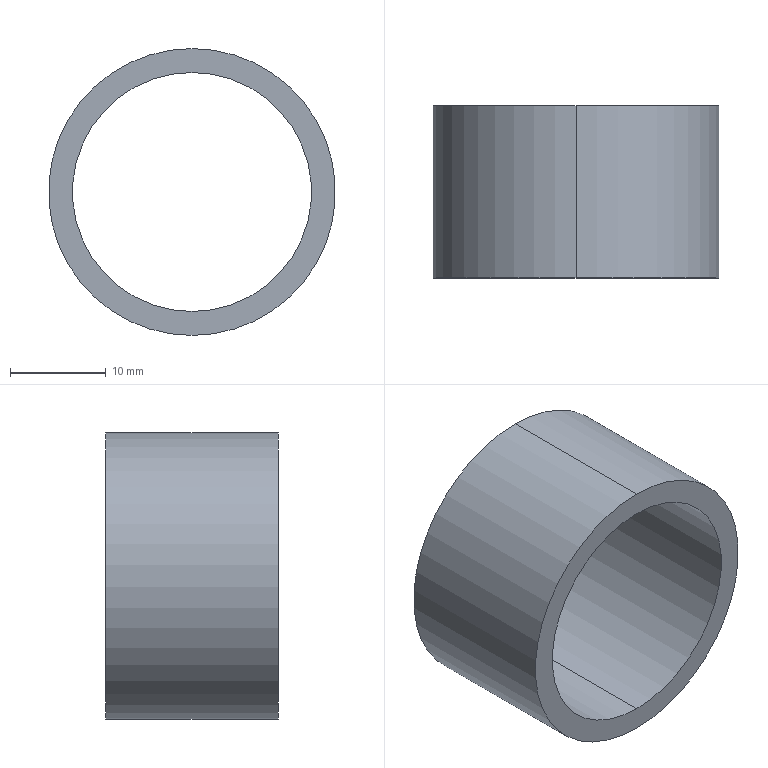Part | SolidWorks | features Extrusion 1 | 1 solid | 6 faces | box 30 x 18 x 30 mm | volume 3888 mm3 | cylinder 4 | plane 2 | commonest cylinder face diameters 25 x2 30 x2
STEP:
#1=CARTESIAN_POINT('',(0.,18.,-12.5));
#2=VERTEX_POINT('',#1);
#3=CARTESIAN_POINT('',(0.,18.,12.5));
#4=VERTEX_POINT('',#3);
#5=CARTESIAN_POINT('',(0.,18.,0.));
#6=DIRECTION('',(0.,1.,0.));
#7=DIRECTION('',(0.,0.,1.));
#8=AXIS2_PLACEMENT_3D('',#5,#6,#7);
#9=CIRCLE('',#8,12.5);
#10=EDGE_CURVE('',#2,#4,#9,.T.);
#11=ORIENTED_EDGE('',*,*,#10,.T.);
#12=CARTESIAN_POINT('',(0.,0.,12.5));
#13=VERTEX_POINT('',#12);
#14=CARTESIAN_POINT('',(0.,18.,12.5));
#15=DIRECTION('',(0.,-1.,0.));
#16=VECTOR('',#15,1000.);
#17=LINE('',#14,#16);
#18=EDGE_CURVE('',#4,#13,#17,.T.);
#19=ORIENTED_EDGE('',*,*,#18,.T.);
#20=CARTESIAN_POINT('',(0.,0.,-12.5));
#21=VERTEX_POINT('',#20);
#22=CARTESIAN_POINT('',(0.,0.,0.));
#23=DIRECTION('',(0.,1.,0.));
#24=DIRECTION('',(0.,0.,1.));
#25=AXIS2_PLACEMENT_3D('',#22,#23,#24);
#26=CIRCLE('',#25,12.5);
#27=EDGE_CURVE('',#21,#13,#26,.T.);
#28=ORIENTED_EDGE('',*,*,#27,.F.);
#29=CARTESIAN_POINT('',(0.,18.,-12.5));
#30=DIRECTION('',(0.,-1.,0.));
#31=VECTOR('',#30,1000.);
#32=LINE('',#29,#31);
#33=EDGE_CURVE('',#2,#21,#32,.T.);
#34=ORIENTED_EDGE('',*,*,#33,.F.);
#35=EDGE_LOOP('',(#11,#19,#28,#34));
#36=FACE_OUTER_BOUND('',#35,.T.);
#37=CARTESIAN_POINT('',(0.,18.,0.));
#38=DIRECTION('',(0.,-1.,0.));
#39=DIRECTION('',(0.,0.,-1.));
#40=AXIS2_PLACEMENT_3D('',#37,#38,#39);
#41=CYLINDRICAL_SURFACE('',#40,12.5);
#42=ADVANCED_FACE('',(#36),#41,.F.);
#43=CARTESIAN_POINT('',(0.,18.,15.));
#44=VERTEX_POINT('',#43);
#45=CARTESIAN_POINT('',(0.,18.,-15.));
#46=VERTEX_POINT('',#45);
#47=CARTESIAN_POINT('',(0.,18.,0.));
#48=DIRECTION('',(0.,1.,0.));
#49=DIRECTION('',(0.,0.,1.));
#50=AXIS2_PLACEMENT_3D('',#47,#48,#49);
#51=CIRCLE('',#50,15.);
#52=EDGE_CURVE('',#44,#46,#51,.T.);
#53=ORIENTED_EDGE('',*,*,#52,.F.);
#54=CARTESIAN_POINT('',(0.,0.,15.));
#55=VERTEX_POINT('',#54);
#56=CARTESIAN_POINT('',(0.,18.,15.));
#57=DIRECTION('',(0.,-1.,0.));
#58=VECTOR('',#57,1000.);
#59=LINE('',#56,#58);
#60=EDGE_CURVE('',#44,#55,#59,.T.);
#61=ORIENTED_EDGE('',*,*,#60,.T.);
#62=CARTESIAN_POINT('',(0.,0.,-15.));
#63=VERTEX_POINT('',#62);
#64=CARTESIAN_POINT('',(0.,0.,0.));
#65=DIRECTION('',(0.,1.,0.));
#66=DIRECTION('',(0.,0.,1.));
#67=AXIS2_PLACEMENT_3D('',#64,#65,#66);
#68=CIRCLE('',#67,15.);
#69=EDGE_CURVE('',#55,#63,#68,.T.);
#70=ORIENTED_EDGE('',*,*,#69,.T.);
#71=CARTESIAN_POINT('',(0.,18.,-15.));
#72=DIRECTION('',(0.,-1.,0.));
#73=VECTOR('',#72,1000.);
#74=LINE('',#71,#73);
#75=EDGE_CURVE('',#46,#63,#74,.T.);
#76=ORIENTED_EDGE('',*,*,#75,.F.);
#77=EDGE_LOOP('',(#53,#61,#70,#76));
#78=FACE_OUTER_BOUND('',#77,.T.);
#79=CARTESIAN_POINT('',(0.,18.,0.));
#80=DIRECTION('',(0.,-1.,0.));
#81=DIRECTION('',(0.,0.,-1.));
#82=AXIS2_PLACEMENT_3D('',#79,#80,#81);
#83=CYLINDRICAL_SURFACE('',#82,15.);
#84=ADVANCED_FACE('',(#78),#83,.T.);
#85=CARTESIAN_POINT('',(0.,18.,0.));
#86=DIRECTION('',(0.,1.,0.));
#87=DIRECTION('',(0.,0.,1.));
#88=AXIS2_PLACEMENT_3D('',#85,#86,#87);
#89=CIRCLE('',#88,15.);
#90=EDGE_CURVE('',#46,#44,#89,.T.);
#91=ORIENTED_EDGE('',*,*,#90,.T.);
#92=ORIENTED_EDGE('',*,*,#52,.T.);
#93=EDGE_LOOP('',(#91,#92));
#94=FACE_OUTER_BOUND('',#93,.T.);
#95=ORIENTED_EDGE('',*,*,#10,.F.);
#96=CARTESIAN_POINT('',(0.,18.,0.));
#97=DIRECTION('',(0.,1.,0.));
#98=DIRECTION('',(0.,0.,1.));
#99=AXIS2_PLACEMENT_3D('',#96,#97,#98);
#100=CIRCLE('',#99,12.5);
#101=EDGE_CURVE('',#4,#2,#100,.T.);
#102=ORIENTED_EDGE('',*,*,#101,.F.);
#103=EDGE_LOOP('',(#95,#102));
#104=FACE_BOUND('',#103,.T.);
#105=CARTESIAN_POINT('',(0.,18.,0.));
#106=DIRECTION('',(0.,1.,0.));
#107=DIRECTION('',(0.,0.,1.));
#108=AXIS2_PLACEMENT_3D('',#105,#106,#107);
#109=PLANE('',#108);
#110=ADVANCED_FACE('',(#94,#104),#109,.T.);
#111=CARTESIAN_POINT('',(0.,0.,0.));
#112=DIRECTION('',(0.,1.,0.));
#113=DIRECTION('',(0.,0.,1.));
#114=AXIS2_PLACEMENT_3D('',#111,#112,#113);
#115=CIRCLE('',#114,15.);
#116=EDGE_CURVE('',#63,#55,#115,.T.);
#117=ORIENTED_EDGE('',*,*,#116,.F.);
#118=ORIENTED_EDGE('',*,*,#69,.F.);
#119=EDGE_LOOP('',(#117,#118));
#120=FACE_OUTER_BOUND('',#119,.T.);
#121=ORIENTED_EDGE('',*,*,#27,.T.);
#122=CARTESIAN_POINT('',(0.,0.,0.));
#123=DIRECTION('',(0.,1.,0.));
#124=DIRECTION('',(0.,0.,1.));
#125=AXIS2_PLACEMENT_3D('',#122,#123,#124);
#126=CIRCLE('',#125,12.5);
#127=EDGE_CURVE('',#13,#21,#126,.T.);
#128=ORIENTED_EDGE('',*,*,#127,.T.);
#129=EDGE_LOOP('',(#121,#128));
#130=FACE_BOUND('',#129,.T.);
#131=CARTESIAN_POINT('',(0.,0.,0.));
#132=DIRECTION('',(0.,1.,0.));
#133=DIRECTION('',(0.,0.,1.));
#134=AXIS2_PLACEMENT_3D('',#131,#132,#133);
#135=PLANE('',#134);
#136=ADVANCED_FACE('',(#120,#130),#135,.F.);
#137=ORIENTED_EDGE('',*,*,#60,.F.);
#138=ORIENTED_EDGE('',*,*,#90,.F.);
#139=ORIENTED_EDGE('',*,*,#75,.T.);
#140=ORIENTED_EDGE('',*,*,#116,.T.);
#141=EDGE_LOOP('',(#137,#138,#139,#140));
#142=FACE_OUTER_BOUND('',#141,.T.);
#143=CARTESIAN_POINT('',(0.,18.,0.));
#144=DIRECTION('',(0.,-1.,0.));
#145=DIRECTION('',(0.,0.,-1.));
#146=AXIS2_PLACEMENT_3D('',#143,#144,#145);
#147=CYLINDRICAL_SURFACE('',#146,15.);
#148=ADVANCED_FACE('',(#142),#147,.T.);
#149=ORIENTED_EDGE('',*,*,#18,.F.);
#150=ORIENTED_EDGE('',*,*,#101,.T.);
#151=ORIENTED_EDGE('',*,*,#33,.T.);
#152=ORIENTED_EDGE('',*,*,#127,.F.);
#153=EDGE_LOOP('',(#149,#150,#151,#152));
#154=FACE_OUTER_BOUND('',#153,.T.);
#155=CARTESIAN_POINT('',(0.,18.,0.));
#156=DIRECTION('',(0.,-1.,0.));
#157=DIRECTION('',(0.,0.,-1.));
#158=AXIS2_PLACEMENT_3D('',#155,#156,#157);
#159=CYLINDRICAL_SURFACE('',#158,12.5);
#160=ADVANCED_FACE('',(#154),#159,.F.);
#161=CLOSED_SHELL('',(#42,#84,#110,#136,#148,#160));
#162=MANIFOLD_SOLID_BREP('',#161);
#163=CARTESIAN_POINT('',(0.,0.,0.));
#164=DIRECTION('',(0.,0.,1.));
#165=DIRECTION('',(1.,0.,0.));
#166=AXIS2_PLACEMENT_3D('',#163,#164,#165);
#167=(LENGTH_UNIT()NAMED_UNIT(*)SI_UNIT(.MILLI.,.METRE.));
#168=UNCERTAINTY_MEASURE_WITH_UNIT(LENGTH_MEASURE(0.00001),#167,'','');
#169=(NAMED_UNIT(*)PLANE_ANGLE_UNIT()SI_UNIT($,.RADIAN.));
#170=(NAMED_UNIT(*)SI_UNIT($,.STERADIAN.)SOLID_ANGLE_UNIT());
#171=(GEOMETRIC_REPRESENTATION_CONTEXT(3)GLOBAL_UNCERTAINTY_ASSIGNED_CONTEXT((#168))GLOBAL_UNIT_ASSIGNED_CONTEXT((#167,#169,#170))REPRESENTATION_CONTEXT('',''));
#172=ADVANCED_BREP_SHAPE_REPRESENTATION('',(#162,#166),#171);